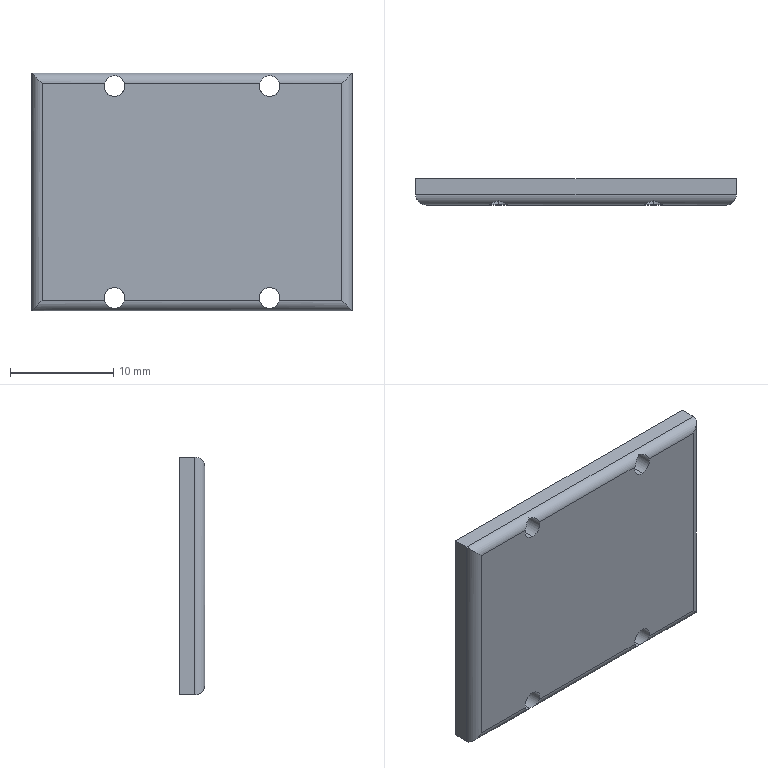Part | SolidWorks | features BaseBody 1 | 1 solid | 18 faces | box 31 x 2.5 x 23 mm | volume 1729 mm3 | cylinder 12 | plane 6 | commonest cylinder face diameters 2 x12
STEP:
#1=CARTESIAN_POINT('',(-7.5,2.5,11.25));
#2=VERTEX_POINT('',#1);
#3=CARTESIAN_POINT('',(-7.5,2.5,9.25));
#4=VERTEX_POINT('',#3);
#5=CARTESIAN_POINT('',(-7.5,2.5,10.25));
#6=DIRECTION('',(0.,-1.,0.));
#7=DIRECTION('',(0.,0.,-1.));
#8=AXIS2_PLACEMENT_3D('',#5,#6,#7);
#9=CIRCLE('',#8,1.);
#10=EDGE_CURVE('',#2,#4,#9,.T.);
#11=ORIENTED_EDGE('',*,*,#10,.F.);
#12=CARTESIAN_POINT('',(-7.5,0.3386,11.25));
#13=VERTEX_POINT('',#12);
#14=CARTESIAN_POINT('',(-7.5,2.5,11.25));
#15=DIRECTION('',(0.,-1.,0.));
#16=VECTOR('',#15,1000.);
#17=LINE('',#14,#16);
#18=EDGE_CURVE('',#2,#13,#17,.T.);
#19=ORIENTED_EDGE('',*,*,#18,.T.);
#20=CARTESIAN_POINT('',(-8.468,0.,10.5));
#21=VERTEX_POINT('',#20);
#22=CARTESIAN_POINT('',(-8.468,0.,10.5));
#23=CARTESIAN_POINT('',(-8.411,0.,10.723));
#24=CARTESIAN_POINT('',(-8.278,0.07612,10.912));
#25=CARTESIAN_POINT('',(-8.027,0.2012,11.107));
#26=CARTESIAN_POINT('',(-7.933,0.2454,11.158));
#27=CARTESIAN_POINT('',(-7.728,0.3144,11.23));
#28=CARTESIAN_POINT('',(-7.615,0.3386,11.25));
#29=CARTESIAN_POINT('',(-7.5,0.3386,11.25));
#30=B_SPLINE_CURVE_WITH_KNOTS('',3,(#22,#23,#24,#25,#26,#27,#28,#29),.UNSPECIFIED.,.F.,.F.,(4,2,2,4),(-0.001355,-0.0006775,-0.0003388,0.),.UNSPECIFIED.);
#31=EDGE_CURVE('',#21,#13,#30,.T.);
#32=ORIENTED_EDGE('',*,*,#31,.F.);
#33=CARTESIAN_POINT('',(-7.5,0.,9.25));
#34=VERTEX_POINT('',#33);
#35=CARTESIAN_POINT('',(-7.5,0.,10.25));
#36=DIRECTION('',(0.,1.,0.));
#37=DIRECTION('',(0.,0.,-1.));
#38=AXIS2_PLACEMENT_3D('',#35,#36,#37);
#39=CIRCLE('',#38,1.);
#40=EDGE_CURVE('',#34,#21,#39,.T.);
#41=ORIENTED_EDGE('',*,*,#40,.F.);
#42=CARTESIAN_POINT('',(-7.5,2.5,9.25));
#43=DIRECTION('',(0.,-1.,0.));
#44=VECTOR('',#43,1000.);
#45=LINE('',#42,#44);
#46=EDGE_CURVE('',#4,#34,#45,.T.);
#47=ORIENTED_EDGE('',*,*,#46,.F.);
#48=EDGE_LOOP('',(#11,#19,#32,#41,#47));
#49=FACE_OUTER_BOUND('',#48,.T.);
#50=CARTESIAN_POINT('',(-7.5,2.5,10.25));
#51=DIRECTION('',(0.,-1.,0.));
#52=DIRECTION('',(0.,0.,-1.));
#53=AXIS2_PLACEMENT_3D('',#50,#51,#52);
#54=CYLINDRICAL_SURFACE('',#53,1.);
#55=ADVANCED_FACE('',(#49),#54,.F.);
#56=CARTESIAN_POINT('',(7.5,2.5,-9.25));
#57=VERTEX_POINT('',#56);
#58=CARTESIAN_POINT('',(7.5,2.5,-11.25));
#59=VERTEX_POINT('',#58);
#60=CARTESIAN_POINT('',(7.5,2.5,-10.25));
#61=DIRECTION('',(0.,-1.,0.));
#62=DIRECTION('',(0.,0.,-1.));
#63=AXIS2_PLACEMENT_3D('',#60,#61,#62);
#64=CIRCLE('',#63,1.);
#65=EDGE_CURVE('',#57,#59,#64,.T.);
#66=ORIENTED_EDGE('',*,*,#65,.F.);
#67=CARTESIAN_POINT('',(7.5,0.,-9.25));
#68=VERTEX_POINT('',#67);
#69=CARTESIAN_POINT('',(7.5,2.5,-9.25));
#70=DIRECTION('',(0.,-1.,0.));
#71=VECTOR('',#70,1000.);
#72=LINE('',#69,#71);
#73=EDGE_CURVE('',#57,#68,#72,.T.);
#74=ORIENTED_EDGE('',*,*,#73,.T.);
#75=CARTESIAN_POINT('',(6.532,0.,-10.5));
#76=VERTEX_POINT('',#75);
#77=CARTESIAN_POINT('',(7.5,0.,-10.25));
#78=DIRECTION('',(0.,1.,0.));
#79=DIRECTION('',(0.,0.,-1.));
#80=AXIS2_PLACEMENT_3D('',#77,#78,#79);
#81=CIRCLE('',#80,1.);
#82=EDGE_CURVE('',#76,#68,#81,.T.);
#83=ORIENTED_EDGE('',*,*,#82,.F.);
#84=CARTESIAN_POINT('',(7.5,0.3386,-11.25));
#85=VERTEX_POINT('',#84);
#86=CARTESIAN_POINT('',(7.5,0.3386,-11.25));
#87=CARTESIAN_POINT('',(7.384,0.3386,-11.25));
#88=CARTESIAN_POINT('',(7.273,0.3147,-11.23));
#89=CARTESIAN_POINT('',(7.068,0.2455,-11.158));
#90=CARTESIAN_POINT('',(6.974,0.2018,-11.107));
#91=CARTESIAN_POINT('',(6.806,0.118,-10.978));
#92=CARTESIAN_POINT('',(6.732,0.07825,-10.9));
#93=CARTESIAN_POINT('',(6.608,0.01882,-10.716));
#94=CARTESIAN_POINT('',(6.561,0.,-10.612));
#95=CARTESIAN_POINT('',(6.532,0.,-10.5));
#96=B_SPLINE_CURVE_WITH_KNOTS('',3,(#86,#87,#88,#89,#90,#91,#92,#93,#94,#95),.UNSPECIFIED.,.F.,.F.,(4,2,2,2,4),(0.,0.0003398,0.0006796,0.001019,0.001359),.UNSPECIFIED.);
#97=EDGE_CURVE('',#85,#76,#96,.T.);
#98=ORIENTED_EDGE('',*,*,#97,.F.);
#99=CARTESIAN_POINT('',(7.5,2.5,-11.25));
#100=DIRECTION('',(0.,-1.,0.));
#101=VECTOR('',#100,1000.);
#102=LINE('',#99,#101);
#103=EDGE_CURVE('',#59,#85,#102,.T.);
#104=ORIENTED_EDGE('',*,*,#103,.F.);
#105=EDGE_LOOP('',(#66,#74,#83,#98,#104));
#106=FACE_OUTER_BOUND('',#105,.T.);
#107=CARTESIAN_POINT('',(7.5,2.5,-10.25));
#108=DIRECTION('',(0.,-1.,0.));
#109=DIRECTION('',(0.,0.,-1.));
#110=AXIS2_PLACEMENT_3D('',#107,#108,#109);
#111=CYLINDRICAL_SURFACE('',#110,1.);
#112=ADVANCED_FACE('',(#106),#111,.F.);
#113=CARTESIAN_POINT('',(-7.5,2.5,-9.25));
#114=VERTEX_POINT('',#113);
#115=CARTESIAN_POINT('',(-7.5,2.5,-11.25));
#116=VERTEX_POINT('',#115);
#117=CARTESIAN_POINT('',(-7.5,2.5,-10.25));
#118=DIRECTION('',(0.,-1.,0.));
#119=DIRECTION('',(0.,0.,-1.));
#120=AXIS2_PLACEMENT_3D('',#117,#118,#119);
#121=CIRCLE('',#120,1.);
#122=EDGE_CURVE('',#114,#116,#121,.T.);
#123=ORIENTED_EDGE('',*,*,#122,.F.);
#124=CARTESIAN_POINT('',(-7.5,0.,-9.25));
#125=VERTEX_POINT('',#124);
#126=CARTESIAN_POINT('',(-7.5,2.5,-9.25));
#127=DIRECTION('',(0.,-1.,0.));
#128=VECTOR('',#127,1000.);
#129=LINE('',#126,#128);
#130=EDGE_CURVE('',#114,#125,#129,.T.);
#131=ORIENTED_EDGE('',*,*,#130,.T.);
#132=CARTESIAN_POINT('',(-8.468,0.,-10.5));
#133=VERTEX_POINT('',#132);
#134=CARTESIAN_POINT('',(-7.5,0.,-10.25));
#135=DIRECTION('',(0.,1.,0.));
#136=DIRECTION('',(0.,0.,-1.));
#137=AXIS2_PLACEMENT_3D('',#134,#135,#136);
#138=CIRCLE('',#137,1.);
#139=EDGE_CURVE('',#133,#125,#138,.T.);
#140=ORIENTED_EDGE('',*,*,#139,.F.);
#141=CARTESIAN_POINT('',(-7.5,0.3386,-11.25));
#142=VERTEX_POINT('',#141);
#143=CARTESIAN_POINT('',(-7.5,0.3386,-11.25));
#144=CARTESIAN_POINT('',(-7.616,0.3386,-11.25));
#145=CARTESIAN_POINT('',(-7.727,0.3147,-11.23));
#146=CARTESIAN_POINT('',(-7.932,0.2455,-11.158));
#147=CARTESIAN_POINT('',(-8.026,0.2018,-11.107));
#148=CARTESIAN_POINT('',(-8.194,0.118,-10.978));
#149=CARTESIAN_POINT('',(-8.268,0.07825,-10.9));
#150=CARTESIAN_POINT('',(-8.392,0.01882,-10.716));
#151=CARTESIAN_POINT('',(-8.439,0.,-10.612));
#152=CARTESIAN_POINT('',(-8.468,0.,-10.5));
#153=B_SPLINE_CURVE_WITH_KNOTS('',3,(#143,#144,#145,#146,#147,#148,#149,#150,#151,#152),.UNSPECIFIED.,.F.,.F.,(4,2,2,2,4),(0.001359,0.0017,0.002041,0.002381,0.002722),.UNSPECIFIED.);
#154=EDGE_CURVE('',#142,#133,#153,.T.);
#155=ORIENTED_EDGE('',*,*,#154,.F.);
#156=CARTESIAN_POINT('',(-7.5,2.5,-11.25));
#157=DIRECTION('',(0.,-1.,0.));
#158=VECTOR('',#157,1000.);
#159=LINE('',#156,#158);
#160=EDGE_CURVE('',#116,#142,#159,.T.);
#161=ORIENTED_EDGE('',*,*,#160,.F.);
#162=EDGE_LOOP('',(#123,#131,#140,#155,#161));
#163=FACE_OUTER_BOUND('',#162,.T.);
#164=CARTESIAN_POINT('',(-7.5,2.5,-10.25));
#165=DIRECTION('',(0.,-1.,0.));
#166=DIRECTION('',(0.,0.,-1.));
#167=AXIS2_PLACEMENT_3D('',#164,#165,#166);
#168=CYLINDRICAL_SURFACE('',#167,1.);
#169=ADVANCED_FACE('',(#163),#168,.F.);
#170=CARTESIAN_POINT('',(7.5,2.5,11.25));
#171=VERTEX_POINT('',#170);
#172=CARTESIAN_POINT('',(7.5,2.5,9.25));
#173=VERTEX_POINT('',#172);
#174=CARTESIAN_POINT('',(7.5,2.5,10.25));
#175=DIRECTION('',(0.,-1.,0.));
#176=DIRECTION('',(0.,0.,-1.));
#177=AXIS2_PLACEMENT_3D('',#174,#175,#176);
#178=CIRCLE('',#177,1.);
#179=EDGE_CURVE('',#171,#173,#178,.T.);
#180=ORIENTED_EDGE('',*,*,#179,.F.);
#181=CARTESIAN_POINT('',(7.5,0.3386,11.25));
#182=VERTEX_POINT('',#181);
#183=CARTESIAN_POINT('',(7.5,2.5,11.25));
#184=DIRECTION('',(0.,-1.,0.));
#185=VECTOR('',#184,1000.);
#186=LINE('',#183,#185);
#187=EDGE_CURVE('',#171,#182,#186,.T.);
#188=ORIENTED_EDGE('',*,*,#187,.T.);
#189=CARTESIAN_POINT('',(6.532,0.,10.5));
#190=VERTEX_POINT('',#189);
#191=CARTESIAN_POINT('',(6.532,0.,10.5));
#192=CARTESIAN_POINT('',(6.589,0.,10.723));
#193=CARTESIAN_POINT('',(6.722,0.07612,10.912));
#194=CARTESIAN_POINT('',(6.973,0.2012,11.107));
#195=CARTESIAN_POINT('',(7.067,0.2454,11.158));
#196=CARTESIAN_POINT('',(7.272,0.3144,11.23));
#197=CARTESIAN_POINT('',(7.385,0.3386,11.25));
#198=CARTESIAN_POINT('',(7.5,0.3386,11.25));
#199=B_SPLINE_CURVE_WITH_KNOTS('',3,(#191,#192,#193,#194,#195,#196,#197,#198),.UNSPECIFIED.,.F.,.F.,(4,2,2,4),(-0.001355,-0.0006775,-0.0003388,0.),.UNSPECIFIED.);
#200=EDGE_CURVE('',#190,#182,#199,.T.);
#201=ORIENTED_EDGE('',*,*,#200,.F.);
#202=CARTESIAN_POINT('',(7.5,0.,9.25));
#203=VERTEX_POINT('',#202);
#204=CARTESIAN_POINT('',(7.5,0.,10.25));
#205=DIRECTION('',(0.,1.,0.));
#206=DIRECTION('',(0.,0.,-1.));
#207=AXIS2_PLACEMENT_3D('',#204,#205,#206);
#208=CIRCLE('',#207,1.);
#209=EDGE_CURVE('',#203,#190,#208,.T.);
#210=ORIENTED_EDGE('',*,*,#209,.F.);
#211=CARTESIAN_POINT('',(7.5,2.5,9.25));
#212=DIRECTION('',(0.,-1.,0.));
#213=VECTOR('',#212,1000.);
#214=LINE('',#211,#213);
#215=EDGE_CURVE('',#173,#203,#214,.T.);
#216=ORIENTED_EDGE('',*,*,#215,.F.);
#217=EDGE_LOOP('',(#180,#188,#201,#210,#216));
#218=FACE_OUTER_BOUND('',#217,.T.);
#219=CARTESIAN_POINT('',(7.5,2.5,10.25));
#220=DIRECTION('',(0.,-1.,0.));
#221=DIRECTION('',(0.,0.,-1.));
#222=AXIS2_PLACEMENT_3D('',#219,#220,#221);
#223=CYLINDRICAL_SURFACE('',#222,1.);
#224=ADVANCED_FACE('',(#218),#223,.F.);
#225=CARTESIAN_POINT('',(-7.5,2.5,10.25));
#226=DIRECTION('',(0.,-1.,0.));
#227=DIRECTION('',(0.,0.,-1.));
#228=AXIS2_PLACEMENT_3D('',#225,#226,#227);
#229=CIRCLE('',#228,1.);
#230=EDGE_CURVE('',#4,#2,#229,.T.);
#231=ORIENTED_EDGE('',*,*,#230,.T.);
#232=ORIENTED_EDGE('',*,*,#10,.T.);
#233=EDGE_LOOP('',(#231,#232));
#234=FACE_BOUND('',#233,.T.);
#235=CARTESIAN_POINT('',(7.5,2.5,-10.25));
#236=DIRECTION('',(0.,-1.,0.));
#237=DIRECTION('',(0.,0.,-1.));
#238=AXIS2_PLACEMENT_3D('',#235,#236,#237);
#239=CIRCLE('',#238,1.);
#240=EDGE_CURVE('',#59,#57,#239,.T.);
#241=ORIENTED_EDGE('',*,*,#240,.T.);
#242=ORIENTED_EDGE('',*,*,#65,.T.);
#243=EDGE_LOOP('',(#241,#242));
#244=FACE_BOUND('',#243,.T.);
#245=CARTESIAN_POINT('',(15.5,2.5,11.5));
#246=VERTEX_POINT('',#245);
#247=CARTESIAN_POINT('',(15.5,2.5,-11.5));
#248=VERTEX_POINT('',#247);
#249=CARTESIAN_POINT('',(15.5,2.5,0.));
#250=DIRECTION('',(0.,0.,-1.));
#251=VECTOR('',#250,1000.);
#252=LINE('',#249,#251);
#253=EDGE_CURVE('',#246,#248,#252,.T.);
#254=ORIENTED_EDGE('',*,*,#253,.T.);
#255=CARTESIAN_POINT('',(-15.5,2.5,-11.5));
#256=VERTEX_POINT('',#255);
#257=CARTESIAN_POINT('',(0.,2.5,-11.5));
#258=DIRECTION('',(-1.,0.,0.));
#259=VECTOR('',#258,1000.);
#260=LINE('',#257,#259);
#261=EDGE_CURVE('',#248,#256,#260,.T.);
#262=ORIENTED_EDGE('',*,*,#261,.T.);
#263=CARTESIAN_POINT('',(-15.5,2.5,11.5));
#264=VERTEX_POINT('',#263);
#265=CARTESIAN_POINT('',(-15.5,2.5,0.));
#266=DIRECTION('',(0.,0.,1.));
#267=VECTOR('',#266,1000.);
#268=LINE('',#265,#267);
#269=EDGE_CURVE('',#256,#264,#268,.T.);
#270=ORIENTED_EDGE('',*,*,#269,.T.);
#271=CARTESIAN_POINT('',(0.,2.5,11.5));
#272=DIRECTION('',(1.,0.,0.));
#273=VECTOR('',#272,1000.);
#274=LINE('',#271,#273);
#275=EDGE_CURVE('',#264,#246,#274,.T.);
#276=ORIENTED_EDGE('',*,*,#275,.T.);
#277=EDGE_LOOP('',(#254,#262,#270,#276));
#278=FACE_OUTER_BOUND('',#277,.T.);
#279=CARTESIAN_POINT('',(-7.5,2.5,-10.25));
#280=DIRECTION('',(0.,-1.,0.));
#281=DIRECTION('',(0.,0.,-1.));
#282=AXIS2_PLACEMENT_3D('',#279,#280,#281);
#283=CIRCLE('',#282,1.);
#284=EDGE_CURVE('',#116,#114,#283,.T.);
#285=ORIENTED_EDGE('',*,*,#284,.T.);
#286=ORIENTED_EDGE('',*,*,#122,.T.);
#287=EDGE_LOOP('',(#285,#286));
#288=FACE_BOUND('',#287,.T.);
#289=CARTESIAN_POINT('',(7.5,2.5,10.25));
#290=DIRECTION('',(0.,-1.,0.));
#291=DIRECTION('',(0.,0.,-1.));
#292=AXIS2_PLACEMENT_3D('',#289,#290,#291);
#293=CIRCLE('',#292,1.);
#294=EDGE_CURVE('',#173,#171,#293,.T.);
#295=ORIENTED_EDGE('',*,*,#294,.T.);
#296=ORIENTED_EDGE('',*,*,#179,.T.);
#297=EDGE_LOOP('',(#295,#296));
#298=FACE_BOUND('',#297,.T.);
#299=CARTESIAN_POINT('',(0.,2.5,0.));
#300=DIRECTION('',(0.,1.,0.));
#301=DIRECTION('',(0.,0.,1.));
#302=AXIS2_PLACEMENT_3D('',#299,#300,#301);
#303=PLANE('',#302);
#304=ADVANCED_FACE('',(#234,#244,#278,#288,#298),#303,.T.);
#305=ORIENTED_EDGE('',*,*,#18,.F.);
#306=ORIENTED_EDGE('',*,*,#230,.F.);
#307=ORIENTED_EDGE('',*,*,#46,.T.);
#308=CARTESIAN_POINT('',(-6.532,0.,10.5));
#309=VERTEX_POINT('',#308);
#310=CARTESIAN_POINT('',(-7.5,0.,10.25));
#311=DIRECTION('',(0.,1.,0.));
#312=DIRECTION('',(0.,0.,-1.));
#313=AXIS2_PLACEMENT_3D('',#310,#311,#312);
#314=CIRCLE('',#313,1.);
#315=EDGE_CURVE('',#309,#34,#314,.T.);
#316=ORIENTED_EDGE('',*,*,#315,.F.);
#317=CARTESIAN_POINT('',(-7.5,0.3386,11.25));
#318=CARTESIAN_POINT('',(-7.384,0.3386,11.25));
#319=CARTESIAN_POINT('',(-7.273,0.3147,11.23));
#320=CARTESIAN_POINT('',(-7.068,0.2455,11.158));
#321=CARTESIAN_POINT('',(-6.974,0.2018,11.107));
#322=CARTESIAN_POINT('',(-6.806,0.118,10.978));
#323=CARTESIAN_POINT('',(-6.732,0.07825,10.9));
#324=CARTESIAN_POINT('',(-6.608,0.01882,10.716));
#325=CARTESIAN_POINT('',(-6.561,0.,10.612));
#326=CARTESIAN_POINT('',(-6.532,0.,10.5));
#327=B_SPLINE_CURVE_WITH_KNOTS('',3,(#317,#318,#319,#320,#321,#322,#323,#324,#325,#326),.UNSPECIFIED.,.F.,.F.,(4,2,2,2,4),(0.,0.0003398,0.0006796,0.001019,0.001359),.UNSPECIFIED.);
#328=EDGE_CURVE('',#13,#309,#327,.T.);
#329=ORIENTED_EDGE('',*,*,#328,.F.);
#330=EDGE_LOOP('',(#305,#306,#307,#316,#329));
#331=FACE_OUTER_BOUND('',#330,.T.);
#332=CARTESIAN_POINT('',(-7.5,2.5,10.25));
#333=DIRECTION('',(0.,-1.,0.));
#334=DIRECTION('',(0.,0.,-1.));
#335=AXIS2_PLACEMENT_3D('',#332,#333,#334);
#336=CYLINDRICAL_SURFACE('',#335,1.);
#337=ADVANCED_FACE('',(#331),#336,.F.);
#338=ORIENTED_EDGE('',*,*,#73,.F.);
#339=ORIENTED_EDGE('',*,*,#240,.F.);
#340=ORIENTED_EDGE('',*,*,#103,.T.);
#341=CARTESIAN_POINT('',(8.468,0.,-10.5));
#342=VERTEX_POINT('',#341);
#343=CARTESIAN_POINT('',(8.468,0.,-10.5));
#344=CARTESIAN_POINT('',(8.411,0.,-10.723));
#345=CARTESIAN_POINT('',(8.278,0.07612,-10.912));
#346=CARTESIAN_POINT('',(8.027,0.2012,-11.107));
#347=CARTESIAN_POINT('',(7.933,0.2454,-11.158));
#348=CARTESIAN_POINT('',(7.728,0.3144,-11.23));
#349=CARTESIAN_POINT('',(7.615,0.3386,-11.25));
#350=CARTESIAN_POINT('',(7.5,0.3386,-11.25));
#351=B_SPLINE_CURVE_WITH_KNOTS('',3,(#343,#344,#345,#346,#347,#348,#349,#350),.UNSPECIFIED.,.F.,.F.,(4,2,2,4),(-0.001355,-0.0006775,-0.0003388,0.),.UNSPECIFIED.);
#352=EDGE_CURVE('',#342,#85,#351,.T.);
#353=ORIENTED_EDGE('',*,*,#352,.F.);
#354=CARTESIAN_POINT('',(7.5,0.,-10.25));
#355=DIRECTION('',(0.,1.,0.));
#356=DIRECTION('',(0.,0.,-1.));
#357=AXIS2_PLACEMENT_3D('',#354,#355,#356);
#358=CIRCLE('',#357,1.);
#359=EDGE_CURVE('',#68,#342,#358,.T.);
#360=ORIENTED_EDGE('',*,*,#359,.F.);
#361=EDGE_LOOP('',(#338,#339,#340,#353,#360));
#362=FACE_OUTER_BOUND('',#361,.T.);
#363=CARTESIAN_POINT('',(7.5,2.5,-10.25));
#364=DIRECTION('',(0.,-1.,0.));
#365=DIRECTION('',(0.,0.,-1.));
#366=AXIS2_PLACEMENT_3D('',#363,#364,#365);
#367=CYLINDRICAL_SURFACE('',#366,1.);
#368=ADVANCED_FACE('',(#362),#367,.F.);
#369=CARTESIAN_POINT('',(-15.5,1.,-11.5));
#370=VERTEX_POINT('',#369);
#371=CARTESIAN_POINT('',(15.5,1.,-11.5));
#372=VERTEX_POINT('',#371);
#373=CARTESIAN_POINT('',(15.5,1.,-11.5));
#374=DIRECTION('',(1.,0.,0.));
#375=VECTOR('',#374,1000.);
#376=LINE('',#373,#375);
#377=EDGE_CURVE('',#370,#372,#376,.T.);
#378=ORIENTED_EDGE('',*,*,#377,.F.);
#379=CARTESIAN_POINT('',(-15.5,2.5,-11.5));
#380=DIRECTION('',(0.,-1.,0.));
#381=VECTOR('',#380,1000.);
#382=LINE('',#379,#381);
#383=EDGE_CURVE('',#256,#370,#382,.T.);
#384=ORIENTED_EDGE('',*,*,#383,.F.);
#385=ORIENTED_EDGE('',*,*,#261,.F.);
#386=CARTESIAN_POINT('',(15.5,2.5,-11.5));
#387=DIRECTION('',(0.,1.,0.));
#388=VECTOR('',#387,1000.);
#389=LINE('',#386,#388);
#390=EDGE_CURVE('',#372,#248,#389,.T.);
#391=ORIENTED_EDGE('',*,*,#390,.F.);
#392=EDGE_LOOP('',(#378,#384,#385,#391));
#393=FACE_OUTER_BOUND('',#392,.T.);
#394=CARTESIAN_POINT('',(15.5,2.5,-11.5));
#395=DIRECTION('',(0.,0.,1.));
#396=DIRECTION('',(1.,0.,0.));
#397=AXIS2_PLACEMENT_3D('',#394,#395,#396);
#398=PLANE('',#397);
#399=ADVANCED_FACE('',(#393),#398,.F.);
#400=CARTESIAN_POINT('',(15.5,1.,11.5));
#401=VERTEX_POINT('',#400);
#402=CARTESIAN_POINT('',(15.5,1.,11.5));
#403=DIRECTION('',(0.,0.,1.));
#404=VECTOR('',#403,1000.);
#405=LINE('',#402,#404);
#406=EDGE_CURVE('',#372,#401,#405,.T.);
#407=ORIENTED_EDGE('',*,*,#406,.F.);
#408=ORIENTED_EDGE('',*,*,#390,.T.);
#409=ORIENTED_EDGE('',*,*,#253,.F.);
#410=CARTESIAN_POINT('',(15.5,2.5,11.5));
#411=DIRECTION('',(0.,1.,0.));
#412=VECTOR('',#411,1000.);
#413=LINE('',#410,#412);
#414=EDGE_CURVE('',#401,#246,#413,.T.);
#415=ORIENTED_EDGE('',*,*,#414,.F.);
#416=EDGE_LOOP('',(#407,#408,#409,#415));
#417=FACE_OUTER_BOUND('',#416,.T.);
#418=CARTESIAN_POINT('',(15.5,2.5,11.5));
#419=DIRECTION('',(-1.,0.,0.));
#420=DIRECTION('',(0.,0.,1.));
#421=AXIS2_PLACEMENT_3D('',#418,#419,#420);
#422=PLANE('',#421);
#423=ADVANCED_FACE('',(#417),#422,.F.);
#424=CARTESIAN_POINT('',(-15.5,1.,11.5));
#425=VERTEX_POINT('',#424);
#426=CARTESIAN_POINT('',(15.5,1.,11.5));
#427=DIRECTION('',(-1.,0.,0.));
#428=VECTOR('',#427,1000.);
#429=LINE('',#426,#428);
#430=EDGE_CURVE('',#401,#425,#429,.T.);
#431=ORIENTED_EDGE('',*,*,#430,.F.);
#432=ORIENTED_EDGE('',*,*,#414,.T.);
#433=ORIENTED_EDGE('',*,*,#275,.F.);
#434=CARTESIAN_POINT('',(-15.5,2.5,11.5));
#435=DIRECTION('',(0.,1.,0.));
#436=VECTOR('',#435,1000.);
#437=LINE('',#434,#436);
#438=EDGE_CURVE('',#425,#264,#437,.T.);
#439=ORIENTED_EDGE('',*,*,#438,.F.);
#440=EDGE_LOOP('',(#431,#432,#433,#439));
#441=FACE_OUTER_BOUND('',#440,.T.);
#442=CARTESIAN_POINT('',(15.5,2.5,11.5));
#443=DIRECTION('',(0.,0.,-1.));
#444=DIRECTION('',(-1.,0.,0.));
#445=AXIS2_PLACEMENT_3D('',#442,#443,#444);
#446=PLANE('',#445);
#447=ADVANCED_FACE('',(#441),#446,.F.);
#448=CARTESIAN_POINT('',(-15.5,1.,11.5));
#449=DIRECTION('',(0.,0.,-1.));
#450=VECTOR('',#449,1000.);
#451=LINE('',#448,#450);
#452=EDGE_CURVE('',#425,#370,#451,.T.);
#453=ORIENTED_EDGE('',*,*,#452,.F.);
#454=ORIENTED_EDGE('',*,*,#438,.T.);
#455=ORIENTED_EDGE('',*,*,#269,.F.);
#456=ORIENTED_EDGE('',*,*,#383,.T.);
#457=EDGE_LOOP('',(#453,#454,#455,#456));
#458=FACE_OUTER_BOUND('',#457,.T.);
#459=CARTESIAN_POINT('',(-15.5,2.5,11.5));
#460=DIRECTION('',(1.,0.,0.));
#461=DIRECTION('',(0.,0.,-1.));
#462=AXIS2_PLACEMENT_3D('',#459,#460,#461);
#463=PLANE('',#462);
#464=ADVANCED_FACE('',(#458),#463,.F.);
#465=ORIENTED_EDGE('',*,*,#130,.F.);
#466=ORIENTED_EDGE('',*,*,#284,.F.);
#467=ORIENTED_EDGE('',*,*,#160,.T.);
#468=CARTESIAN_POINT('',(-6.532,0.,-10.5));
#469=VERTEX_POINT('',#468);
#470=CARTESIAN_POINT('',(-6.532,0.,-10.5));
#471=CARTESIAN_POINT('',(-6.589,0.,-10.723));
#472=CARTESIAN_POINT('',(-6.722,0.07612,-10.912));
#473=CARTESIAN_POINT('',(-6.973,0.2012,-11.107));
#474=CARTESIAN_POINT('',(-7.067,0.2454,-11.158));
#475=CARTESIAN_POINT('',(-7.272,0.3144,-11.23));
#476=CARTESIAN_POINT('',(-7.385,0.3386,-11.25));
#477=CARTESIAN_POINT('',(-7.5,0.3386,-11.25));
#478=B_SPLINE_CURVE_WITH_KNOTS('',3,(#470,#471,#472,#473,#474,#475,#476,#477),.UNSPECIFIED.,.F.,.F.,(4,2,2,4),(0.,0.0006795,0.001019,0.001359),.UNSPECIFIED.);
#479=EDGE_CURVE('',#469,#142,#478,.T.);
#480=ORIENTED_EDGE('',*,*,#479,.F.);
#481=CARTESIAN_POINT('',(-7.5,0.,-10.25));
#482=DIRECTION('',(0.,1.,0.));
#483=DIRECTION('',(0.,0.,-1.));
#484=AXIS2_PLACEMENT_3D('',#481,#482,#483);
#485=CIRCLE('',#484,1.);
#486=EDGE_CURVE('',#125,#469,#485,.T.);
#487=ORIENTED_EDGE('',*,*,#486,.F.);
#488=EDGE_LOOP('',(#465,#466,#467,#480,#487));
#489=FACE_OUTER_BOUND('',#488,.T.);
#490=CARTESIAN_POINT('',(-7.5,2.5,-10.25));
#491=DIRECTION('',(0.,-1.,0.));
#492=DIRECTION('',(0.,0.,-1.));
#493=AXIS2_PLACEMENT_3D('',#490,#491,#492);
#494=CYLINDRICAL_SURFACE('',#493,1.);
#495=ADVANCED_FACE('',(#489),#494,.F.);
#496=ORIENTED_EDGE('',*,*,#187,.F.);
#497=ORIENTED_EDGE('',*,*,#294,.F.);
#498=ORIENTED_EDGE('',*,*,#215,.T.);
#499=CARTESIAN_POINT('',(8.468,0.,10.5));
#500=VERTEX_POINT('',#499);
#501=CARTESIAN_POINT('',(7.5,0.,10.25));
#502=DIRECTION('',(0.,1.,0.));
#503=DIRECTION('',(0.,0.,-1.));
#504=AXIS2_PLACEMENT_3D('',#501,#502,#503);
#505=CIRCLE('',#504,1.);
#506=EDGE_CURVE('',#500,#203,#505,.T.);
#507=ORIENTED_EDGE('',*,*,#506,.F.);
#508=CARTESIAN_POINT('',(7.5,0.3386,11.25));
#509=CARTESIAN_POINT('',(7.616,0.3386,11.25));
#510=CARTESIAN_POINT('',(7.727,0.3147,11.23));
#511=CARTESIAN_POINT('',(7.932,0.2455,11.158));
#512=CARTESIAN_POINT('',(8.026,0.2018,11.107));
#513=CARTESIAN_POINT('',(8.194,0.118,10.978));
#514=CARTESIAN_POINT('',(8.268,0.07825,10.9));
#515=CARTESIAN_POINT('',(8.392,0.01882,10.716));
#516=CARTESIAN_POINT('',(8.439,0.,10.612));
#517=CARTESIAN_POINT('',(8.468,0.,10.5));
#518=B_SPLINE_CURVE_WITH_KNOTS('',3,(#508,#509,#510,#511,#512,#513,#514,#515,#516,#517),.UNSPECIFIED.,.F.,.F.,(4,2,2,2,4),(0.,0.0003398,0.0006796,0.001019,0.001359),.UNSPECIFIED.);
#519=EDGE_CURVE('',#182,#500,#518,.T.);
#520=ORIENTED_EDGE('',*,*,#519,.F.);
#521=EDGE_LOOP('',(#496,#497,#498,#507,#520));
#522=FACE_OUTER_BOUND('',#521,.T.);
#523=CARTESIAN_POINT('',(7.5,2.5,10.25));
#524=DIRECTION('',(0.,-1.,0.));
#525=DIRECTION('',(0.,0.,-1.));
#526=AXIS2_PLACEMENT_3D('',#523,#524,#525);
#527=CYLINDRICAL_SURFACE('',#526,1.);
#528=ADVANCED_FACE('',(#522),#527,.F.);
#529=ORIENTED_EDGE('',*,*,#506,.T.);
#530=ORIENTED_EDGE('',*,*,#209,.T.);
#531=CARTESIAN_POINT('',(0.,0.,10.5));
#532=DIRECTION('',(1.,0.,0.));
#533=VECTOR('',#532,1000.);
#534=LINE('',#531,#533);
#535=EDGE_CURVE('',#309,#190,#534,.T.);
#536=ORIENTED_EDGE('',*,*,#535,.F.);
#537=ORIENTED_EDGE('',*,*,#315,.T.);
#538=ORIENTED_EDGE('',*,*,#40,.T.);
#539=CARTESIAN_POINT('',(-14.5,0.,10.5));
#540=VERTEX_POINT('',#539);
#541=CARTESIAN_POINT('',(0.,0.,10.5));
#542=DIRECTION('',(1.,0.,0.));
#543=VECTOR('',#542,1000.);
#544=LINE('',#541,#543);
#545=EDGE_CURVE('',#540,#21,#544,.T.);
#546=ORIENTED_EDGE('',*,*,#545,.F.);
#547=CARTESIAN_POINT('',(-14.5,0.,-10.5));
#548=VERTEX_POINT('',#547);
#549=CARTESIAN_POINT('',(-14.5,0.,0.));
#550=DIRECTION('',(0.,0.,1.));
#551=VECTOR('',#550,1000.);
#552=LINE('',#549,#551);
#553=EDGE_CURVE('',#548,#540,#552,.T.);
#554=ORIENTED_EDGE('',*,*,#553,.F.);
#555=CARTESIAN_POINT('',(0.,0.,-10.5));
#556=DIRECTION('',(-1.,0.,0.));
#557=VECTOR('',#556,1000.);
#558=LINE('',#555,#557);
#559=EDGE_CURVE('',#133,#548,#558,.T.);
#560=ORIENTED_EDGE('',*,*,#559,.F.);
#561=ORIENTED_EDGE('',*,*,#139,.T.);
#562=ORIENTED_EDGE('',*,*,#486,.T.);
#563=CARTESIAN_POINT('',(0.,0.,-10.5));
#564=DIRECTION('',(-1.,0.,0.));
#565=VECTOR('',#564,1000.);
#566=LINE('',#563,#565);
#567=EDGE_CURVE('',#76,#469,#566,.T.);
#568=ORIENTED_EDGE('',*,*,#567,.F.);
#569=ORIENTED_EDGE('',*,*,#82,.T.);
#570=ORIENTED_EDGE('',*,*,#359,.T.);
#571=CARTESIAN_POINT('',(14.5,0.,-10.5));
#572=VERTEX_POINT('',#571);
#573=CARTESIAN_POINT('',(0.,0.,-10.5));
#574=DIRECTION('',(-1.,0.,0.));
#575=VECTOR('',#574,1000.);
#576=LINE('',#573,#575);
#577=EDGE_CURVE('',#572,#342,#576,.T.);
#578=ORIENTED_EDGE('',*,*,#577,.F.);
#579=CARTESIAN_POINT('',(14.5,0.,10.5));
#580=VERTEX_POINT('',#579);
#581=CARTESIAN_POINT('',(14.5,0.,0.));
#582=DIRECTION('',(0.,0.,-1.));
#583=VECTOR('',#582,1000.);
#584=LINE('',#581,#583);
#585=EDGE_CURVE('',#580,#572,#584,.T.);
#586=ORIENTED_EDGE('',*,*,#585,.F.);
#587=CARTESIAN_POINT('',(0.,0.,10.5));
#588=DIRECTION('',(1.,0.,0.));
#589=VECTOR('',#588,1000.);
#590=LINE('',#587,#589);
#591=EDGE_CURVE('',#500,#580,#590,.T.);
#592=ORIENTED_EDGE('',*,*,#591,.F.);
#593=EDGE_LOOP('',(#529,#530,#536,#537,#538,#546,#554,#560,#561,#562,#568,#569,#570,#578,#586,#592));
#594=FACE_OUTER_BOUND('',#593,.T.);
#595=CARTESIAN_POINT('',(0.,0.,0.));
#596=DIRECTION('',(0.,1.,0.));
#597=DIRECTION('',(0.,0.,1.));
#598=AXIS2_PLACEMENT_3D('',#595,#596,#597);
#599=PLANE('',#598);
#600=ADVANCED_FACE('',(#594),#599,.F.);
#601=ORIENTED_EDGE('',*,*,#567,.T.);
#602=ORIENTED_EDGE('',*,*,#479,.T.);
#603=ORIENTED_EDGE('',*,*,#154,.T.);
#604=ORIENTED_EDGE('',*,*,#559,.T.);
#605=CARTESIAN_POINT('',(-14.5,0.,-10.5));
#606=CARTESIAN_POINT('',(-15.086,0.,-11.086));
#607=CARTESIAN_POINT('',(-15.5,0.4142,-11.5));
#608=CARTESIAN_POINT('',(-15.5,1.,-11.5));
#609=(BOUNDED_CURVE()B_SPLINE_CURVE(3,(#605,#606,#607,#608),.UNSPECIFIED.,.F.,.F.)B_SPLINE_CURVE_WITH_KNOTS((4,4),(4.712,6.283),.UNSPECIFIED.)CURVE()GEOMETRIC_REPRESENTATION_ITEM()RATIONAL_B_SPLINE_CURVE((1.,0.8047,0.8047,1.))REPRESENTATION_ITEM(''));
#610=EDGE_CURVE('',#548,#370,#609,.T.);
#611=ORIENTED_EDGE('',*,*,#610,.T.);
#612=ORIENTED_EDGE('',*,*,#377,.T.);
#613=CARTESIAN_POINT('',(15.5,1.,-11.5));
#614=CARTESIAN_POINT('',(15.5,0.4142,-11.5));
#615=CARTESIAN_POINT('',(15.086,0.,-11.086));
#616=CARTESIAN_POINT('',(14.5,0.,-10.5));
#617=(BOUNDED_CURVE()B_SPLINE_CURVE(3,(#613,#614,#615,#616),.UNSPECIFIED.,.F.,.F.)B_SPLINE_CURVE_WITH_KNOTS((4,4),(3.142,4.712),.UNSPECIFIED.)CURVE()GEOMETRIC_REPRESENTATION_ITEM()RATIONAL_B_SPLINE_CURVE((1.,0.8047,0.8047,1.))REPRESENTATION_ITEM(''));
#618=EDGE_CURVE('',#372,#572,#617,.T.);
#619=ORIENTED_EDGE('',*,*,#618,.T.);
#620=ORIENTED_EDGE('',*,*,#577,.T.);
#621=ORIENTED_EDGE('',*,*,#352,.T.);
#622=ORIENTED_EDGE('',*,*,#97,.T.);
#623=EDGE_LOOP('',(#601,#602,#603,#604,#611,#612,#619,#620,#621,#622));
#624=FACE_OUTER_BOUND('',#623,.T.);
#625=CARTESIAN_POINT('',(15.5,1.,-10.5));
#626=DIRECTION('',(-1.,0.,0.));
#627=DIRECTION('',(0.,0.,1.));
#628=AXIS2_PLACEMENT_3D('',#625,#626,#627);
#629=CYLINDRICAL_SURFACE('',#628,1.);
#630=ADVANCED_FACE('',(#624),#629,.T.);
#631=CARTESIAN_POINT('',(15.5,1.,11.5));
#632=CARTESIAN_POINT('',(15.5,0.4142,11.5));
#633=CARTESIAN_POINT('',(15.086,0.,11.086));
#634=CARTESIAN_POINT('',(14.5,0.,10.5));
#635=(BOUNDED_CURVE()B_SPLINE_CURVE(3,(#631,#632,#633,#634),.UNSPECIFIED.,.F.,.F.)B_SPLINE_CURVE_WITH_KNOTS((4,4),(3.142,4.712),.UNSPECIFIED.)CURVE()GEOMETRIC_REPRESENTATION_ITEM()RATIONAL_B_SPLINE_CURVE((1.,0.8047,0.8047,1.))REPRESENTATION_ITEM(''));
#636=EDGE_CURVE('',#401,#580,#635,.T.);
#637=ORIENTED_EDGE('',*,*,#636,.T.);
#638=ORIENTED_EDGE('',*,*,#585,.T.);
#639=ORIENTED_EDGE('',*,*,#618,.F.);
#640=ORIENTED_EDGE('',*,*,#406,.T.);
#641=EDGE_LOOP('',(#637,#638,#639,#640));
#642=FACE_OUTER_BOUND('',#641,.T.);
#643=CARTESIAN_POINT('',(14.5,1.,11.5));
#644=DIRECTION('',(0.,0.,-1.));
#645=DIRECTION('',(-1.,0.,0.));
#646=AXIS2_PLACEMENT_3D('',#643,#644,#645);
#647=CYLINDRICAL_SURFACE('',#646,1.);
#648=ADVANCED_FACE('',(#642),#647,.T.);
#649=ORIENTED_EDGE('',*,*,#535,.T.);
#650=ORIENTED_EDGE('',*,*,#200,.T.);
#651=ORIENTED_EDGE('',*,*,#519,.T.);
#652=ORIENTED_EDGE('',*,*,#591,.T.);
#653=ORIENTED_EDGE('',*,*,#636,.F.);
#654=ORIENTED_EDGE('',*,*,#430,.T.);
#655=CARTESIAN_POINT('',(-15.5,1.,11.5));
#656=CARTESIAN_POINT('',(-15.5,0.4142,11.5));
#657=CARTESIAN_POINT('',(-15.086,0.,11.086));
#658=CARTESIAN_POINT('',(-14.5,0.,10.5));
#659=(BOUNDED_CURVE()B_SPLINE_CURVE(3,(#655,#656,#657,#658),.UNSPECIFIED.,.F.,.F.)B_SPLINE_CURVE_WITH_KNOTS((4,4),(3.142,4.712),.UNSPECIFIED.)CURVE()GEOMETRIC_REPRESENTATION_ITEM()RATIONAL_B_SPLINE_CURVE((1.,0.8047,0.8047,1.))REPRESENTATION_ITEM(''));
#660=EDGE_CURVE('',#425,#540,#659,.T.);
#661=ORIENTED_EDGE('',*,*,#660,.T.);
#662=ORIENTED_EDGE('',*,*,#545,.T.);
#663=ORIENTED_EDGE('',*,*,#31,.T.);
#664=ORIENTED_EDGE('',*,*,#328,.T.);
#665=EDGE_LOOP('',(#649,#650,#651,#652,#653,#654,#661,#662,#663,#664));
#666=FACE_OUTER_BOUND('',#665,.T.);
#667=CARTESIAN_POINT('',(15.5,1.,10.5));
#668=DIRECTION('',(1.,0.,0.));
#669=DIRECTION('',(0.,0.,-1.));
#670=AXIS2_PLACEMENT_3D('',#667,#668,#669);
#671=CYLINDRICAL_SURFACE('',#670,1.);
#672=ADVANCED_FACE('',(#666),#671,.T.);
#673=ORIENTED_EDGE('',*,*,#660,.F.);
#674=ORIENTED_EDGE('',*,*,#452,.T.);
#675=ORIENTED_EDGE('',*,*,#610,.F.);
#676=ORIENTED_EDGE('',*,*,#553,.T.);
#677=EDGE_LOOP('',(#673,#674,#675,#676));
#678=FACE_OUTER_BOUND('',#677,.T.);
#679=CARTESIAN_POINT('',(-14.5,1.,11.5));
#680=DIRECTION('',(0.,0.,1.));
#681=DIRECTION('',(1.,0.,0.));
#682=AXIS2_PLACEMENT_3D('',#679,#680,#681);
#683=CYLINDRICAL_SURFACE('',#682,1.);
#684=ADVANCED_FACE('',(#678),#683,.T.);
#685=CLOSED_SHELL('',(#55,#112,#169,#224,#304,#337,#368,#399,#423,#447,#464,#495,#528,#600,#630,#648,#672,#684));
#686=MANIFOLD_SOLID_BREP('',#685);
#687=CARTESIAN_POINT('',(0.,0.,0.));
#688=DIRECTION('',(0.,0.,1.));
#689=DIRECTION('',(1.,0.,0.));
#690=AXIS2_PLACEMENT_3D('',#687,#688,#689);
#691=(LENGTH_UNIT()NAMED_UNIT(*)SI_UNIT(.MILLI.,.METRE.));
#692=UNCERTAINTY_MEASURE_WITH_UNIT(LENGTH_MEASURE(0.00001),#691,'','');
#693=(NAMED_UNIT(*)PLANE_ANGLE_UNIT()SI_UNIT($,.RADIAN.));
#694=(NAMED_UNIT(*)SI_UNIT($,.STERADIAN.)SOLID_ANGLE_UNIT());
#695=(GEOMETRIC_REPRESENTATION_CONTEXT(3)GLOBAL_UNCERTAINTY_ASSIGNED_CONTEXT((#692))GLOBAL_UNIT_ASSIGNED_CONTEXT((#691,#693,#694))REPRESENTATION_CONTEXT('',''));
#696=ADVANCED_BREP_SHAPE_REPRESENTATION('',(#686,#690),#695);